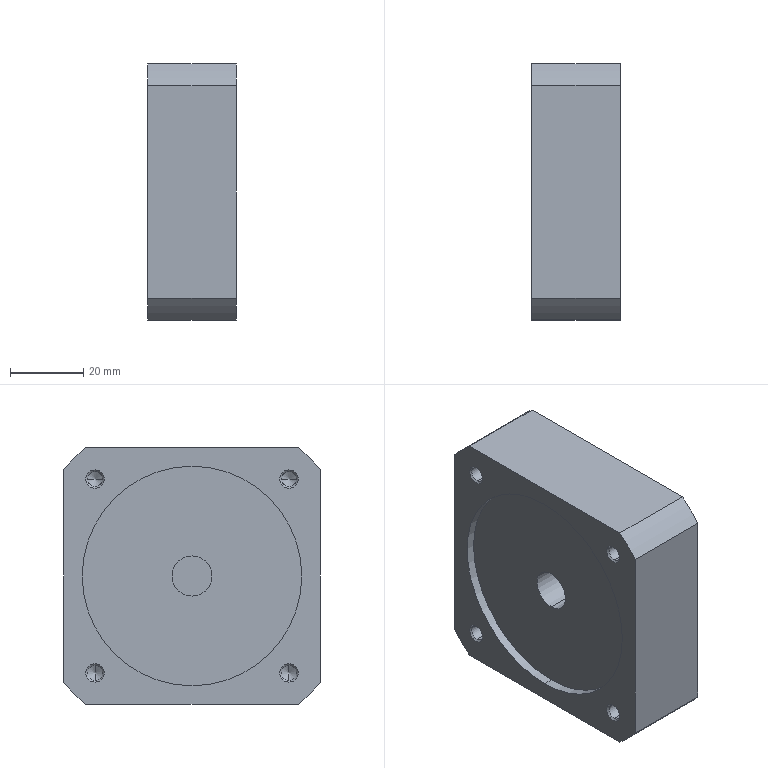Part | STEP file | _PLE60-5_MOTOR-OP2 (intermediate flanges 11-23-60-75-5-70-2.5) | 1 solid | 43 faces | box 24.2 x 70 x 70 mm | volume 107278 mm3 | cylinder 18 | cone 16 | plane 9 | commonest cylinder face diameters 4.134 x8 91 x4 7 x2 11 x2 60 x2
STEP:
#1=CARTESIAN_POINT('',(8.,34.5,5.5));
#2=VERTEX_POINT('',#1);
#3=CARTESIAN_POINT('',(8.,34.5,12.5));
#4=VERTEX_POINT('',#3);
#5=CARTESIAN_POINT('',(8.,34.5,9.));
#6=DIRECTION('',(0.,1.,0.));
#7=DIRECTION('',(0.,0.,1.));
#8=AXIS2_PLACEMENT_3D('',#5,#6,#7);
#9=CIRCLE('',#8,3.5);
#10=EDGE_CURVE('',#2,#4,#9,.T.);
#11=ORIENTED_EDGE('',*,*,#10,.F.);
#12=CARTESIAN_POINT('',(8.,35.,5.5));
#13=VERTEX_POINT('',#12);
#14=CARTESIAN_POINT('',(8.,34.5,5.5));
#15=DIRECTION('',(0.,1.,0.));
#16=VECTOR('',#15,1000.);
#17=LINE('',#14,#16);
#18=EDGE_CURVE('',#2,#13,#17,.T.);
#19=ORIENTED_EDGE('',*,*,#18,.T.);
#20=CARTESIAN_POINT('',(8.,35.,12.5));
#21=VERTEX_POINT('',#20);
#22=CARTESIAN_POINT('',(8.,35.,9.));
#23=DIRECTION('',(0.,1.,0.));
#24=DIRECTION('',(0.,0.,1.));
#25=AXIS2_PLACEMENT_3D('',#22,#23,#24);
#26=CIRCLE('',#25,3.5);
#27=EDGE_CURVE('',#13,#21,#26,.T.);
#28=ORIENTED_EDGE('',*,*,#27,.T.);
#29=CARTESIAN_POINT('',(8.,34.5,12.5));
#30=DIRECTION('',(0.,1.,0.));
#31=VECTOR('',#30,1000.);
#32=LINE('',#29,#31);
#33=EDGE_CURVE('',#4,#21,#32,.T.);
#34=ORIENTED_EDGE('',*,*,#33,.F.);
#35=EDGE_LOOP('',(#11,#19,#28,#34));
#36=FACE_OUTER_BOUND('',#35,.T.);
#37=CARTESIAN_POINT('',(8.,34.5,9.));
#38=DIRECTION('',(0.,1.,0.));
#39=DIRECTION('',(0.,0.,1.));
#40=AXIS2_PLACEMENT_3D('',#37,#38,#39);
#41=CYLINDRICAL_SURFACE('',#40,3.5);
#42=ADVANCED_FACE('',(#36),#41,.F.);
#43=CARTESIAN_POINT('',(2.5,0.,-30.));
#44=VERTEX_POINT('',#43);
#45=CARTESIAN_POINT('',(2.5,0.,30.));
#46=VERTEX_POINT('',#45);
#47=CARTESIAN_POINT('',(2.5,0.,0.));
#48=DIRECTION('',(-1.,0.,0.));
#49=DIRECTION('',(0.,0.,1.));
#50=AXIS2_PLACEMENT_3D('',#47,#48,#49);
#51=CIRCLE('',#50,30.);
#52=EDGE_CURVE('',#44,#46,#51,.T.);
#53=ORIENTED_EDGE('',*,*,#52,.F.);
#54=CARTESIAN_POINT('',(0.,0.,-30.));
#55=VERTEX_POINT('',#54);
#56=CARTESIAN_POINT('',(23.,0.,-30.));
#57=DIRECTION('',(-1.,0.,0.));
#58=VECTOR('',#57,1000.);
#59=LINE('',#56,#58);
#60=EDGE_CURVE('',#44,#55,#59,.T.);
#61=ORIENTED_EDGE('',*,*,#60,.T.);
#62=CARTESIAN_POINT('',(0.,0.,30.));
#63=VERTEX_POINT('',#62);
#64=CARTESIAN_POINT('',(0.,0.,0.));
#65=DIRECTION('',(-1.,0.,0.));
#66=DIRECTION('',(0.,0.,1.));
#67=AXIS2_PLACEMENT_3D('',#64,#65,#66);
#68=CIRCLE('',#67,30.);
#69=EDGE_CURVE('',#55,#63,#68,.T.);
#70=ORIENTED_EDGE('',*,*,#69,.T.);
#71=CARTESIAN_POINT('',(23.,0.,30.));
#72=DIRECTION('',(-1.,0.,0.));
#73=VECTOR('',#72,1000.);
#74=LINE('',#71,#73);
#75=EDGE_CURVE('',#46,#63,#74,.T.);
#76=ORIENTED_EDGE('',*,*,#75,.F.);
#77=EDGE_LOOP('',(#53,#61,#70,#76));
#78=FACE_OUTER_BOUND('',#77,.T.);
#79=CARTESIAN_POINT('',(23.,0.,0.));
#80=DIRECTION('',(-1.,0.,0.));
#81=DIRECTION('',(0.,0.,1.));
#82=AXIS2_PLACEMENT_3D('',#79,#80,#81);
#83=CYLINDRICAL_SURFACE('',#82,30.);
#84=ADVANCED_FACE('',(#78),#83,.F.);
#85=CARTESIAN_POINT('',(0.433,26.517,-28.584));
#86=VERTEX_POINT('',#85);
#87=CARTESIAN_POINT('',(0.433,26.517,-24.45));
#88=VERTEX_POINT('',#87);
#89=CARTESIAN_POINT('',(0.433,26.517,-26.517));
#90=DIRECTION('',(-1.,0.,0.));
#91=DIRECTION('',(0.,0.,1.));
#92=AXIS2_PLACEMENT_3D('',#89,#90,#91);
#93=CIRCLE('',#92,2.067);
#94=EDGE_CURVE('',#86,#88,#93,.T.);
#95=ORIENTED_EDGE('',*,*,#94,.F.);
#96=CARTESIAN_POINT('',(0.,26.517,-29.017));
#97=VERTEX_POINT('',#96);
#98=CARTESIAN_POINT('',(0.,26.517,-29.017));
#99=DIRECTION('',(-0.7071,0.,-0.7071));
#100=VECTOR('',#99,1000.);
#101=LINE('',#98,#100);
#102=EDGE_CURVE('',#86,#97,#101,.T.);
#103=ORIENTED_EDGE('',*,*,#102,.T.);
#104=CARTESIAN_POINT('',(0.,26.517,-24.017));
#105=VERTEX_POINT('',#104);
#106=CARTESIAN_POINT('',(0.,26.517,-26.517));
#107=DIRECTION('',(-1.,0.,0.));
#108=DIRECTION('',(0.,0.,1.));
#109=AXIS2_PLACEMENT_3D('',#106,#107,#108);
#110=CIRCLE('',#109,2.5);
#111=EDGE_CURVE('',#97,#105,#110,.T.);
#112=ORIENTED_EDGE('',*,*,#111,.T.);
#113=CARTESIAN_POINT('',(0.,26.517,-24.017));
#114=DIRECTION('',(-0.7071,0.,0.7071));
#115=VECTOR('',#114,1000.);
#116=LINE('',#113,#115);
#117=EDGE_CURVE('',#88,#105,#116,.T.);
#118=ORIENTED_EDGE('',*,*,#117,.F.);
#119=EDGE_LOOP('',(#95,#103,#112,#118));
#120=FACE_OUTER_BOUND('',#119,.T.);
#121=CARTESIAN_POINT('',(0.,26.517,-26.517));
#122=DIRECTION('',(-1.,0.,0.));
#123=DIRECTION('',(0.,0.,1.));
#124=AXIS2_PLACEMENT_3D('',#121,#122,#123);
#125=CONICAL_SURFACE('',#124,2.5,0.7854);
#126=ADVANCED_FACE('',(#120),#125,.F.);
#127=CARTESIAN_POINT('',(0.433,-26.517,-28.584));
#128=VERTEX_POINT('',#127);
#129=CARTESIAN_POINT('',(0.433,-26.517,-24.45));
#130=VERTEX_POINT('',#129);
#131=CARTESIAN_POINT('',(0.433,-26.517,-26.517));
#132=DIRECTION('',(-1.,0.,0.));
#133=DIRECTION('',(0.,0.,1.));
#134=AXIS2_PLACEMENT_3D('',#131,#132,#133);
#135=CIRCLE('',#134,2.067);
#136=EDGE_CURVE('',#128,#130,#135,.T.);
#137=ORIENTED_EDGE('',*,*,#136,.F.);
#138=CARTESIAN_POINT('',(0.,-26.517,-29.017));
#139=VERTEX_POINT('',#138);
#140=CARTESIAN_POINT('',(0.,-26.517,-29.017));
#141=DIRECTION('',(-0.7071,0.,-0.7071));
#142=VECTOR('',#141,1000.);
#143=LINE('',#140,#142);
#144=EDGE_CURVE('',#128,#139,#143,.T.);
#145=ORIENTED_EDGE('',*,*,#144,.T.);
#146=CARTESIAN_POINT('',(0.,-26.517,-24.017));
#147=VERTEX_POINT('',#146);
#148=CARTESIAN_POINT('',(0.,-26.517,-26.517));
#149=DIRECTION('',(-1.,0.,0.));
#150=DIRECTION('',(0.,0.,1.));
#151=AXIS2_PLACEMENT_3D('',#148,#149,#150);
#152=CIRCLE('',#151,2.5);
#153=EDGE_CURVE('',#139,#147,#152,.T.);
#154=ORIENTED_EDGE('',*,*,#153,.T.);
#155=CARTESIAN_POINT('',(0.,-26.517,-24.017));
#156=DIRECTION('',(-0.7071,0.,0.7071));
#157=VECTOR('',#156,1000.);
#158=LINE('',#155,#157);
#159=EDGE_CURVE('',#130,#147,#158,.T.);
#160=ORIENTED_EDGE('',*,*,#159,.F.);
#161=EDGE_LOOP('',(#137,#145,#154,#160));
#162=FACE_OUTER_BOUND('',#161,.T.);
#163=CARTESIAN_POINT('',(0.,-26.517,-26.517));
#164=DIRECTION('',(-1.,0.,0.));
#165=DIRECTION('',(0.,0.,1.));
#166=AXIS2_PLACEMENT_3D('',#163,#164,#165);
#167=CONICAL_SURFACE('',#166,2.5,0.7854);
#168=ADVANCED_FACE('',(#162),#167,.F.);
#169=CARTESIAN_POINT('',(0.433,-26.517,24.45));
#170=VERTEX_POINT('',#169);
#171=CARTESIAN_POINT('',(0.433,-26.517,28.584));
#172=VERTEX_POINT('',#171);
#173=CARTESIAN_POINT('',(0.433,-26.517,26.517));
#174=DIRECTION('',(-1.,0.,0.));
#175=DIRECTION('',(0.,0.,1.));
#176=AXIS2_PLACEMENT_3D('',#173,#174,#175);
#177=CIRCLE('',#176,2.067);
#178=EDGE_CURVE('',#170,#172,#177,.T.);
#179=ORIENTED_EDGE('',*,*,#178,.F.);
#180=CARTESIAN_POINT('',(0.,-26.517,24.017));
#181=VERTEX_POINT('',#180);
#182=CARTESIAN_POINT('',(0.,-26.517,24.017));
#183=DIRECTION('',(-0.7071,0.,-0.7071));
#184=VECTOR('',#183,1000.);
#185=LINE('',#182,#184);
#186=EDGE_CURVE('',#170,#181,#185,.T.);
#187=ORIENTED_EDGE('',*,*,#186,.T.);
#188=CARTESIAN_POINT('',(0.,-26.517,29.017));
#189=VERTEX_POINT('',#188);
#190=CARTESIAN_POINT('',(0.,-26.517,26.517));
#191=DIRECTION('',(-1.,0.,0.));
#192=DIRECTION('',(0.,0.,1.));
#193=AXIS2_PLACEMENT_3D('',#190,#191,#192);
#194=CIRCLE('',#193,2.5);
#195=EDGE_CURVE('',#181,#189,#194,.T.);
#196=ORIENTED_EDGE('',*,*,#195,.T.);
#197=CARTESIAN_POINT('',(0.,-26.517,29.017));
#198=DIRECTION('',(-0.7071,0.,0.7071));
#199=VECTOR('',#198,1000.);
#200=LINE('',#197,#199);
#201=EDGE_CURVE('',#172,#189,#200,.T.);
#202=ORIENTED_EDGE('',*,*,#201,.F.);
#203=EDGE_LOOP('',(#179,#187,#196,#202));
#204=FACE_OUTER_BOUND('',#203,.T.);
#205=CARTESIAN_POINT('',(0.,-26.517,26.517));
#206=DIRECTION('',(-1.,0.,0.));
#207=DIRECTION('',(0.,0.,1.));
#208=AXIS2_PLACEMENT_3D('',#205,#206,#207);
#209=CONICAL_SURFACE('',#208,2.5,0.7854);
#210=ADVANCED_FACE('',(#204),#209,.F.);
#211=CARTESIAN_POINT('',(0.433,26.517,24.45));
#212=VERTEX_POINT('',#211);
#213=CARTESIAN_POINT('',(0.433,26.517,28.584));
#214=VERTEX_POINT('',#213);
#215=CARTESIAN_POINT('',(0.433,26.517,26.517));
#216=DIRECTION('',(-1.,0.,0.));
#217=DIRECTION('',(0.,0.,1.));
#218=AXIS2_PLACEMENT_3D('',#215,#216,#217);
#219=CIRCLE('',#218,2.067);
#220=EDGE_CURVE('',#212,#214,#219,.T.);
#221=ORIENTED_EDGE('',*,*,#220,.F.);
#222=CARTESIAN_POINT('',(0.,26.517,24.017));
#223=VERTEX_POINT('',#222);
#224=CARTESIAN_POINT('',(0.,26.517,24.017));
#225=DIRECTION('',(-0.7071,0.,-0.7071));
#226=VECTOR('',#225,1000.);
#227=LINE('',#224,#226);
#228=EDGE_CURVE('',#212,#223,#227,.T.);
#229=ORIENTED_EDGE('',*,*,#228,.T.);
#230=CARTESIAN_POINT('',(0.,26.517,29.017));
#231=VERTEX_POINT('',#230);
#232=CARTESIAN_POINT('',(0.,26.517,26.517));
#233=DIRECTION('',(-1.,0.,0.));
#234=DIRECTION('',(0.,0.,1.));
#235=AXIS2_PLACEMENT_3D('',#232,#233,#234);
#236=CIRCLE('',#235,2.5);
#237=EDGE_CURVE('',#223,#231,#236,.T.);
#238=ORIENTED_EDGE('',*,*,#237,.T.);
#239=CARTESIAN_POINT('',(0.,26.517,29.017));
#240=DIRECTION('',(-0.7071,0.,0.7071));
#241=VECTOR('',#240,1000.);
#242=LINE('',#239,#241);
#243=EDGE_CURVE('',#214,#231,#242,.T.);
#244=ORIENTED_EDGE('',*,*,#243,.F.);
#245=EDGE_LOOP('',(#221,#229,#238,#244));
#246=FACE_OUTER_BOUND('',#245,.T.);
#247=CARTESIAN_POINT('',(0.,26.517,26.517));
#248=DIRECTION('',(-1.,0.,0.));
#249=DIRECTION('',(0.,0.,1.));
#250=AXIS2_PLACEMENT_3D('',#247,#248,#249);
#251=CONICAL_SURFACE('',#250,2.5,0.7854);
#252=ADVANCED_FACE('',(#246),#251,.F.);
#253=CARTESIAN_POINT('',(12.,26.517,-28.584));
#254=VERTEX_POINT('',#253);
#255=CARTESIAN_POINT('',(12.,26.517,-24.45));
#256=VERTEX_POINT('',#255);
#257=CARTESIAN_POINT('',(12.,26.517,-26.517));
#258=DIRECTION('',(-1.,0.,0.));
#259=DIRECTION('',(0.,0.,1.));
#260=AXIS2_PLACEMENT_3D('',#257,#258,#259);
#261=CIRCLE('',#260,2.067);
#262=EDGE_CURVE('',#254,#256,#261,.T.);
#263=ORIENTED_EDGE('',*,*,#262,.F.);
#264=CARTESIAN_POINT('',(13.193,26.517,-28.584));
#265=DIRECTION('',(-1.,0.,0.));
#266=VECTOR('',#265,1000.);
#267=LINE('',#264,#266);
#268=EDGE_CURVE('',#254,#86,#267,.T.);
#269=ORIENTED_EDGE('',*,*,#268,.T.);
#270=ORIENTED_EDGE('',*,*,#94,.T.);
#271=CARTESIAN_POINT('',(13.193,26.517,-24.45));
#272=DIRECTION('',(-1.,0.,0.));
#273=VECTOR('',#272,1000.);
#274=LINE('',#271,#273);
#275=EDGE_CURVE('',#256,#88,#274,.T.);
#276=ORIENTED_EDGE('',*,*,#275,.F.);
#277=EDGE_LOOP('',(#263,#269,#270,#276));
#278=FACE_OUTER_BOUND('',#277,.T.);
#279=CARTESIAN_POINT('',(13.193,26.517,-26.517));
#280=DIRECTION('',(-1.,0.,0.));
#281=DIRECTION('',(0.,0.,1.));
#282=AXIS2_PLACEMENT_3D('',#279,#280,#281);
#283=CYLINDRICAL_SURFACE('',#282,2.067);
#284=ADVANCED_FACE('',(#278),#283,.F.);
#285=CARTESIAN_POINT('',(12.,-26.517,-28.584));
#286=VERTEX_POINT('',#285);
#287=CARTESIAN_POINT('',(12.,-26.517,-24.45));
#288=VERTEX_POINT('',#287);
#289=CARTESIAN_POINT('',(12.,-26.517,-26.517));
#290=DIRECTION('',(-1.,0.,0.));
#291=DIRECTION('',(0.,0.,1.));
#292=AXIS2_PLACEMENT_3D('',#289,#290,#291);
#293=CIRCLE('',#292,2.067);
#294=EDGE_CURVE('',#286,#288,#293,.T.);
#295=ORIENTED_EDGE('',*,*,#294,.F.);
#296=CARTESIAN_POINT('',(13.193,-26.517,-28.584));
#297=DIRECTION('',(-1.,0.,0.));
#298=VECTOR('',#297,1000.);
#299=LINE('',#296,#298);
#300=EDGE_CURVE('',#286,#128,#299,.T.);
#301=ORIENTED_EDGE('',*,*,#300,.T.);
#302=ORIENTED_EDGE('',*,*,#136,.T.);
#303=CARTESIAN_POINT('',(13.193,-26.517,-24.45));
#304=DIRECTION('',(-1.,0.,0.));
#305=VECTOR('',#304,1000.);
#306=LINE('',#303,#305);
#307=EDGE_CURVE('',#288,#130,#306,.T.);
#308=ORIENTED_EDGE('',*,*,#307,.F.);
#309=EDGE_LOOP('',(#295,#301,#302,#308));
#310=FACE_OUTER_BOUND('',#309,.T.);
#311=CARTESIAN_POINT('',(13.193,-26.517,-26.517));
#312=DIRECTION('',(-1.,0.,0.));
#313=DIRECTION('',(0.,0.,1.));
#314=AXIS2_PLACEMENT_3D('',#311,#312,#313);
#315=CYLINDRICAL_SURFACE('',#314,2.067);
#316=ADVANCED_FACE('',(#310),#315,.F.);
#317=CARTESIAN_POINT('',(12.,-26.517,24.45));
#318=VERTEX_POINT('',#317);
#319=CARTESIAN_POINT('',(12.,-28.584,26.517));
#320=VERTEX_POINT('',#319);
#321=CARTESIAN_POINT('',(12.,-26.517,26.517));
#322=DIRECTION('',(-1.,0.,0.));
#323=DIRECTION('',(0.,0.,1.));
#324=AXIS2_PLACEMENT_3D('',#321,#322,#323);
#325=CIRCLE('',#324,2.067);
#326=EDGE_CURVE('',#318,#320,#325,.T.);
#327=ORIENTED_EDGE('',*,*,#326,.F.);
#328=CARTESIAN_POINT('',(13.193,-26.517,24.45));
#329=DIRECTION('',(-1.,0.,0.));
#330=VECTOR('',#329,1000.);
#331=LINE('',#328,#330);
#332=EDGE_CURVE('',#318,#170,#331,.T.);
#333=ORIENTED_EDGE('',*,*,#332,.T.);
#334=ORIENTED_EDGE('',*,*,#178,.T.);
#335=CARTESIAN_POINT('',(12.,-26.517,28.584));
#336=VERTEX_POINT('',#335);
#337=CARTESIAN_POINT('',(13.193,-26.517,28.584));
#338=DIRECTION('',(-1.,0.,0.));
#339=VECTOR('',#338,1000.);
#340=LINE('',#337,#339);
#341=EDGE_CURVE('',#336,#172,#340,.T.);
#342=ORIENTED_EDGE('',*,*,#341,.F.);
#343=CARTESIAN_POINT('',(12.,-26.517,26.517));
#344=DIRECTION('',(-1.,0.,0.));
#345=DIRECTION('',(0.,0.,1.));
#346=AXIS2_PLACEMENT_3D('',#343,#344,#345);
#347=CIRCLE('',#346,2.067);
#348=EDGE_CURVE('',#320,#336,#347,.T.);
#349=ORIENTED_EDGE('',*,*,#348,.F.);
#350=EDGE_LOOP('',(#327,#333,#334,#342,#349));
#351=FACE_OUTER_BOUND('',#350,.T.);
#352=CARTESIAN_POINT('',(13.193,-26.517,26.517));
#353=DIRECTION('',(-1.,0.,0.));
#354=DIRECTION('',(0.,0.,1.));
#355=AXIS2_PLACEMENT_3D('',#352,#353,#354);
#356=CYLINDRICAL_SURFACE('',#355,2.067);
#357=ADVANCED_FACE('',(#351),#356,.F.);
#358=CARTESIAN_POINT('',(12.,26.517,24.45));
#359=VERTEX_POINT('',#358);
#360=CARTESIAN_POINT('',(12.,24.45,26.517));
#361=VERTEX_POINT('',#360);
#362=CARTESIAN_POINT('',(12.,26.517,26.517));
#363=DIRECTION('',(-1.,0.,0.));
#364=DIRECTION('',(0.,0.,1.));
#365=AXIS2_PLACEMENT_3D('',#362,#363,#364);
#366=CIRCLE('',#365,2.067);
#367=EDGE_CURVE('',#359,#361,#366,.T.);
#368=ORIENTED_EDGE('',*,*,#367,.F.);
#369=CARTESIAN_POINT('',(13.193,26.517,24.45));
#370=DIRECTION('',(-1.,0.,0.));
#371=VECTOR('',#370,1000.);
#372=LINE('',#369,#371);
#373=EDGE_CURVE('',#359,#212,#372,.T.);
#374=ORIENTED_EDGE('',*,*,#373,.T.);
#375=ORIENTED_EDGE('',*,*,#220,.T.);
#376=CARTESIAN_POINT('',(12.,26.517,28.584));
#377=VERTEX_POINT('',#376);
#378=CARTESIAN_POINT('',(13.193,26.517,28.584));
#379=DIRECTION('',(-1.,0.,0.));
#380=VECTOR('',#379,1000.);
#381=LINE('',#378,#380);
#382=EDGE_CURVE('',#377,#214,#381,.T.);
#383=ORIENTED_EDGE('',*,*,#382,.F.);
#384=CARTESIAN_POINT('',(12.,26.517,26.517));
#385=DIRECTION('',(-1.,0.,0.));
#386=DIRECTION('',(0.,0.,1.));
#387=AXIS2_PLACEMENT_3D('',#384,#385,#386);
#388=CIRCLE('',#387,2.067);
#389=EDGE_CURVE('',#361,#377,#388,.T.);
#390=ORIENTED_EDGE('',*,*,#389,.F.);
#391=EDGE_LOOP('',(#368,#374,#375,#383,#390));
#392=FACE_OUTER_BOUND('',#391,.T.);
#393=CARTESIAN_POINT('',(13.193,26.517,26.517));
#394=DIRECTION('',(-1.,0.,0.));
#395=DIRECTION('',(0.,0.,1.));
#396=AXIS2_PLACEMENT_3D('',#393,#394,#395);
#397=CYLINDRICAL_SURFACE('',#396,2.067);
#398=ADVANCED_FACE('',(#392),#397,.F.);
#399=CARTESIAN_POINT('',(23.,0.,-5.5));
#400=VERTEX_POINT('',#399);
#401=CARTESIAN_POINT('',(23.,0.,5.5));
#402=VERTEX_POINT('',#401);
#403=CARTESIAN_POINT('',(23.,0.,0.));
#404=DIRECTION('',(-1.,0.,0.));
#405=DIRECTION('',(0.,0.,1.));
#406=AXIS2_PLACEMENT_3D('',#403,#404,#405);
#407=CIRCLE('',#406,5.5);
#408=EDGE_CURVE('',#400,#402,#407,.T.);
#409=ORIENTED_EDGE('',*,*,#408,.F.);
#410=CARTESIAN_POINT('',(2.5,0.,-5.5));
#411=VERTEX_POINT('',#410);
#412=CARTESIAN_POINT('',(23.,0.,-5.5));
#413=DIRECTION('',(-1.,0.,0.));
#414=VECTOR('',#413,1000.);
#415=LINE('',#412,#414);
#416=EDGE_CURVE('',#400,#411,#415,.T.);
#417=ORIENTED_EDGE('',*,*,#416,.T.);
#418=CARTESIAN_POINT('',(2.5,0.,5.5));
#419=VERTEX_POINT('',#418);
#420=CARTESIAN_POINT('',(2.5,0.,0.));
#421=DIRECTION('',(1.,0.,0.));
#422=DIRECTION('',(0.,0.,1.));
#423=AXIS2_PLACEMENT_3D('',#420,#421,#422);
#424=CIRCLE('',#423,5.5);
#425=EDGE_CURVE('',#419,#411,#424,.T.);
#426=ORIENTED_EDGE('',*,*,#425,.F.);
#427=CARTESIAN_POINT('',(23.,0.,5.5));
#428=DIRECTION('',(-1.,0.,0.));
#429=VECTOR('',#428,1000.);
#430=LINE('',#427,#429);
#431=EDGE_CURVE('',#402,#419,#430,.T.);
#432=ORIENTED_EDGE('',*,*,#431,.F.);
#433=EDGE_LOOP('',(#409,#417,#426,#432));
#434=FACE_OUTER_BOUND('',#433,.T.);
#435=CARTESIAN_POINT('',(23.,0.,0.));
#436=DIRECTION('',(-1.,0.,0.));
#437=DIRECTION('',(0.,0.,1.));
#438=AXIS2_PLACEMENT_3D('',#435,#436,#437);
#439=CYLINDRICAL_SURFACE('',#438,5.5);
#440=ADVANCED_FACE('',(#434),#439,.F.);
#441=CARTESIAN_POINT('',(13.193,26.517,-26.517));
#442=VERTEX_POINT('',#441);
#443=CARTESIAN_POINT('',(12.,26.517,-24.45));
#444=DIRECTION('',(-0.5,0.,0.866));
#445=VECTOR('',#444,1000.);
#446=LINE('',#443,#445);
#447=EDGE_CURVE('',#442,#256,#446,.T.);
#448=ORIENTED_EDGE('',*,*,#447,.F.);
#449=CARTESIAN_POINT('',(12.,26.517,-28.584));
#450=DIRECTION('',(-0.5,0.,-0.866));
#451=VECTOR('',#450,1000.);
#452=LINE('',#449,#451);
#453=EDGE_CURVE('',#442,#254,#452,.T.);
#454=ORIENTED_EDGE('',*,*,#453,.T.);
#455=ORIENTED_EDGE('',*,*,#262,.T.);
#456=EDGE_LOOP('',(#448,#454,#455));
#457=FACE_OUTER_BOUND('',#456,.T.);
#458=CARTESIAN_POINT('',(12.,26.517,-26.517));
#459=DIRECTION('',(-1.,0.,0.));
#460=DIRECTION('',(0.,0.,1.));
#461=AXIS2_PLACEMENT_3D('',#458,#459,#460);
#462=CONICAL_SURFACE('',#461,2.067,1.047);
#463=ADVANCED_FACE('',(#457),#462,.F.);
#464=CARTESIAN_POINT('',(13.193,-26.517,-26.517));
#465=VERTEX_POINT('',#464);
#466=CARTESIAN_POINT('',(12.,-26.517,-24.45));
#467=DIRECTION('',(-0.5,0.,0.866));
#468=VECTOR('',#467,1000.);
#469=LINE('',#466,#468);
#470=EDGE_CURVE('',#465,#288,#469,.T.);
#471=ORIENTED_EDGE('',*,*,#470,.F.);
#472=CARTESIAN_POINT('',(12.,-26.517,-28.584));
#473=DIRECTION('',(-0.5,0.,-0.866));
#474=VECTOR('',#473,1000.);
#475=LINE('',#472,#474);
#476=EDGE_CURVE('',#465,#286,#475,.T.);
#477=ORIENTED_EDGE('',*,*,#476,.T.);
#478=ORIENTED_EDGE('',*,*,#294,.T.);
#479=EDGE_LOOP('',(#471,#477,#478));
#480=FACE_OUTER_BOUND('',#479,.T.);
#481=CARTESIAN_POINT('',(12.,-26.517,-26.517));
#482=DIRECTION('',(-1.,0.,0.));
#483=DIRECTION('',(0.,0.,1.));
#484=AXIS2_PLACEMENT_3D('',#481,#482,#483);
#485=CONICAL_SURFACE('',#484,2.067,1.047);
#486=ADVANCED_FACE('',(#480),#485,.F.);
#487=CARTESIAN_POINT('',(13.193,-26.517,26.517));
#488=VERTEX_POINT('',#487);
#489=CARTESIAN_POINT('',(12.,-28.584,26.517));
#490=DIRECTION('',(-0.5,-0.866,0.));
#491=VECTOR('',#490,1000.);
#492=LINE('',#489,#491);
#493=EDGE_CURVE('',#488,#320,#492,.T.);
#494=ORIENTED_EDGE('',*,*,#493,.F.);
#495=CARTESIAN_POINT('',(12.,-24.45,26.517));
#496=VERTEX_POINT('',#495);
#497=CARTESIAN_POINT('',(12.,-24.45,26.517));
#498=DIRECTION('',(-0.5,0.866,0.));
#499=VECTOR('',#498,1000.);
#500=LINE('',#497,#499);
#501=EDGE_CURVE('',#488,#496,#500,.T.);
#502=ORIENTED_EDGE('',*,*,#501,.T.);
#503=CARTESIAN_POINT('',(12.,-26.517,26.517));
#504=DIRECTION('',(-1.,0.,0.));
#505=DIRECTION('',(0.,0.,1.));
#506=AXIS2_PLACEMENT_3D('',#503,#504,#505);
#507=CIRCLE('',#506,2.067);
#508=EDGE_CURVE('',#496,#318,#507,.T.);
#509=ORIENTED_EDGE('',*,*,#508,.T.);
#510=ORIENTED_EDGE('',*,*,#326,.T.);
#511=EDGE_LOOP('',(#494,#502,#509,#510));
#512=FACE_OUTER_BOUND('',#511,.T.);
#513=CARTESIAN_POINT('',(12.,-26.517,26.517));
#514=DIRECTION('',(-1.,0.,0.));
#515=DIRECTION('',(0.,-1.,0.));
#516=AXIS2_PLACEMENT_3D('',#513,#514,#515);
#517=CONICAL_SURFACE('',#516,2.067,1.047);
#518=ADVANCED_FACE('',(#512),#517,.F.);
#519=CARTESIAN_POINT('',(13.193,26.517,26.517));
#520=VERTEX_POINT('',#519);
#521=CARTESIAN_POINT('',(12.,24.45,26.517));
#522=DIRECTION('',(-0.5,-0.866,0.));
#523=VECTOR('',#522,1000.);
#524=LINE('',#521,#523);
#525=EDGE_CURVE('',#520,#361,#524,.T.);
#526=ORIENTED_EDGE('',*,*,#525,.F.);
#527=CARTESIAN_POINT('',(12.,28.584,26.517));
#528=VERTEX_POINT('',#527);
#529=CARTESIAN_POINT('',(12.,28.584,26.517));
#530=DIRECTION('',(-0.5,0.866,0.));
#531=VECTOR('',#530,1000.);
#532=LINE('',#529,#531);
#533=EDGE_CURVE('',#520,#528,#532,.T.);
#534=ORIENTED_EDGE('',*,*,#533,.T.);
#535=CARTESIAN_POINT('',(12.,26.517,26.517));
#536=DIRECTION('',(-1.,0.,0.));
#537=DIRECTION('',(0.,0.,1.));
#538=AXIS2_PLACEMENT_3D('',#535,#536,#537);
#539=CIRCLE('',#538,2.067);
#540=EDGE_CURVE('',#528,#359,#539,.T.);
#541=ORIENTED_EDGE('',*,*,#540,.T.);
#542=ORIENTED_EDGE('',*,*,#367,.T.);
#543=EDGE_LOOP('',(#526,#534,#541,#542));
#544=FACE_OUTER_BOUND('',#543,.T.);
#545=CARTESIAN_POINT('',(12.,26.517,26.517));
#546=DIRECTION('',(-1.,0.,0.));
#547=DIRECTION('',(0.,-1.,0.));
#548=AXIS2_PLACEMENT_3D('',#545,#546,#547);
#549=CONICAL_SURFACE('',#548,2.067,1.047);
#550=ADVANCED_FACE('',(#544),#549,.F.);
#551=CARTESIAN_POINT('',(24.2,35.,-29.073));
#552=VERTEX_POINT('',#551);
#553=CARTESIAN_POINT('',(24.2,35.,29.073));
#554=VERTEX_POINT('',#553);
#555=CARTESIAN_POINT('',(24.2,35.,0.));
#556=DIRECTION('',(0.,0.,1.));
#557=VECTOR('',#556,1000.);
#558=LINE('',#555,#557);
#559=EDGE_CURVE('',#552,#554,#558,.T.);
#560=ORIENTED_EDGE('',*,*,#559,.T.);
#561=CARTESIAN_POINT('',(24.2,29.073,35.));
#562=VERTEX_POINT('',#561);
#563=CARTESIAN_POINT('',(24.2,0.,0.));
#564=DIRECTION('',(1.,0.,0.));
#565=DIRECTION('',(0.,0.,-1.));
#566=AXIS2_PLACEMENT_3D('',#563,#564,#565);
#567=CIRCLE('',#566,45.5);
#568=EDGE_CURVE('',#554,#562,#567,.T.);
#569=ORIENTED_EDGE('',*,*,#568,.T.);
#570=CARTESIAN_POINT('',(24.2,-29.073,35.));
#571=VERTEX_POINT('',#570);
#572=CARTESIAN_POINT('',(24.2,0.,35.));
#573=DIRECTION('',(0.,-1.,0.));
#574=VECTOR('',#573,1000.);
#575=LINE('',#572,#574);
#576=EDGE_CURVE('',#562,#571,#575,.T.);
#577=ORIENTED_EDGE('',*,*,#576,.T.);
#578=CARTESIAN_POINT('',(24.2,-35.,29.073));
#579=VERTEX_POINT('',#578);
#580=CARTESIAN_POINT('',(24.2,0.,0.));
#581=DIRECTION('',(1.,0.,0.));
#582=DIRECTION('',(0.,0.,-1.));
#583=AXIS2_PLACEMENT_3D('',#580,#581,#582);
#584=CIRCLE('',#583,45.5);
#585=EDGE_CURVE('',#571,#579,#584,.T.);
#586=ORIENTED_EDGE('',*,*,#585,.T.);
#587=CARTESIAN_POINT('',(24.2,-35.,-29.073));
#588=VERTEX_POINT('',#587);
#589=CARTESIAN_POINT('',(24.2,-35.,0.));
#590=DIRECTION('',(0.,0.,-1.));
#591=VECTOR('',#590,1000.);
#592=LINE('',#589,#591);
#593=EDGE_CURVE('',#579,#588,#592,.T.);
#594=ORIENTED_EDGE('',*,*,#593,.T.);
#595=CARTESIAN_POINT('',(24.2,-29.073,-35.));
#596=VERTEX_POINT('',#595);
#597=CARTESIAN_POINT('',(24.2,0.,0.));
#598=DIRECTION('',(1.,0.,0.));
#599=DIRECTION('',(0.,0.,-1.));
#600=AXIS2_PLACEMENT_3D('',#597,#598,#599);
#601=CIRCLE('',#600,45.5);
#602=EDGE_CURVE('',#588,#596,#601,.T.);
#603=ORIENTED_EDGE('',*,*,#602,.T.);
#604=CARTESIAN_POINT('',(24.2,29.073,-35.));
#605=VERTEX_POINT('',#604);
#606=CARTESIAN_POINT('',(24.2,0.,-35.));
#607=DIRECTION('',(0.,1.,0.));
#608=VECTOR('',#607,1000.);
#609=LINE('',#606,#608);
#610=EDGE_CURVE('',#596,#605,#609,.T.);
#611=ORIENTED_EDGE('',*,*,#610,.T.);
#612=CARTESIAN_POINT('',(24.2,0.,0.));
#613=DIRECTION('',(1.,0.,0.));
#614=DIRECTION('',(0.,0.,-1.));
#615=AXIS2_PLACEMENT_3D('',#612,#613,#614);
#616=CIRCLE('',#615,45.5);
#617=EDGE_CURVE('',#605,#552,#616,.T.);
#618=ORIENTED_EDGE('',*,*,#617,.T.);
#619=EDGE_LOOP('',(#560,#569,#577,#586,#594,#603,#611,#618));
#620=FACE_OUTER_BOUND('',#619,.T.);
#621=CARTESIAN_POINT('',(24.2,0.,0.));
#622=DIRECTION('',(1.,0.,0.));
#623=DIRECTION('',(0.,0.,-1.));
#624=AXIS2_PLACEMENT_3D('',#621,#622,#623);
#625=PLANE('',#624);
#626=ADVANCED_FACE('',(#620),#625,.T.);
#627=ORIENTED_EDGE('',*,*,#568,.F.);
#628=CARTESIAN_POINT('',(0.,35.,29.073));
#629=VERTEX_POINT('',#628);
#630=CARTESIAN_POINT('',(24.2,35.,29.073));
#631=DIRECTION('',(-1.,0.,0.));
#632=VECTOR('',#631,1000.);
#633=LINE('',#630,#632);
#634=EDGE_CURVE('',#554,#629,#633,.T.);
#635=ORIENTED_EDGE('',*,*,#634,.T.);
#636=CARTESIAN_POINT('',(0.,29.073,35.));
#637=VERTEX_POINT('',#636);
#638=CARTESIAN_POINT('',(0.,0.,0.));
#639=DIRECTION('',(1.,0.,0.));
#640=DIRECTION('',(0.,0.,-1.));
#641=AXIS2_PLACEMENT_3D('',#638,#639,#640);
#642=CIRCLE('',#641,45.5);
#643=EDGE_CURVE('',#629,#637,#642,.T.);
#644=ORIENTED_EDGE('',*,*,#643,.T.);
#645=CARTESIAN_POINT('',(24.2,29.073,35.));
#646=DIRECTION('',(1.,0.,0.));
#647=VECTOR('',#646,1000.);
#648=LINE('',#645,#647);
#649=EDGE_CURVE('',#637,#562,#648,.T.);
#650=ORIENTED_EDGE('',*,*,#649,.T.);
#651=EDGE_LOOP('',(#627,#635,#644,#650));
#652=FACE_OUTER_BOUND('',#651,.T.);
#653=CARTESIAN_POINT('',(24.2,0.,0.));
#654=DIRECTION('',(1.,0.,0.));
#655=DIRECTION('',(0.,0.,-1.));
#656=AXIS2_PLACEMENT_3D('',#653,#654,#655);
#657=CYLINDRICAL_SURFACE('',#656,45.5);
#658=ADVANCED_FACE('',(#652),#657,.T.);
#659=ORIENTED_EDGE('',*,*,#634,.F.);
#660=ORIENTED_EDGE('',*,*,#559,.F.);
#661=CARTESIAN_POINT('',(0.,35.,-29.073));
#662=VERTEX_POINT('',#661);
#663=CARTESIAN_POINT('',(24.2,35.,-29.073));
#664=DIRECTION('',(1.,0.,0.));
#665=VECTOR('',#664,1000.);
#666=LINE('',#663,#665);
#667=EDGE_CURVE('',#662,#552,#666,.T.);
#668=ORIENTED_EDGE('',*,*,#667,.F.);
#669=CARTESIAN_POINT('',(0.,35.,-29.073));
#670=DIRECTION('',(0.,0.,-1.));
#671=VECTOR('',#670,1000.);
#672=LINE('',#669,#671);
#673=EDGE_CURVE('',#629,#662,#672,.T.);
#674=ORIENTED_EDGE('',*,*,#673,.F.);
#675=EDGE_LOOP('',(#659,#660,#668,#674));
#676=FACE_OUTER_BOUND('',#675,.T.);
#677=CARTESIAN_POINT('',(8.,35.,9.));
#678=DIRECTION('',(0.,1.,0.));
#679=DIRECTION('',(0.,0.,1.));
#680=AXIS2_PLACEMENT_3D('',#677,#678,#679);
#681=CIRCLE('',#680,3.5);
#682=EDGE_CURVE('',#21,#13,#681,.T.);
#683=ORIENTED_EDGE('',*,*,#682,.F.);
#684=ORIENTED_EDGE('',*,*,#27,.F.);
#685=EDGE_LOOP('',(#683,#684));
#686=FACE_BOUND('',#685,.T.);
#687=CARTESIAN_POINT('',(24.2,35.,-29.073));
#688=DIRECTION('',(0.,-1.,0.));
#689=DIRECTION('',(0.,0.,-1.));
#690=AXIS2_PLACEMENT_3D('',#687,#688,#689);
#691=PLANE('',#690);
#692=ADVANCED_FACE('',(#676,#686),#691,.F.);
#693=ORIENTED_EDGE('',*,*,#617,.F.);
#694=CARTESIAN_POINT('',(0.,29.073,-35.));
#695=VERTEX_POINT('',#694);
#696=CARTESIAN_POINT('',(24.2,29.073,-35.));
#697=DIRECTION('',(-1.,0.,0.));
#698=VECTOR('',#697,1000.);
#699=LINE('',#696,#698);
#700=EDGE_CURVE('',#605,#695,#699,.T.);
#701=ORIENTED_EDGE('',*,*,#700,.T.);
#702=CARTESIAN_POINT('',(0.,0.,0.));
#703=DIRECTION('',(1.,0.,0.));
#704=DIRECTION('',(0.,0.,-1.));
#705=AXIS2_PLACEMENT_3D('',#702,#703,#704);
#706=CIRCLE('',#705,45.5);
#707=EDGE_CURVE('',#695,#662,#706,.T.);
#708=ORIENTED_EDGE('',*,*,#707,.T.);
#709=ORIENTED_EDGE('',*,*,#667,.T.);
#710=EDGE_LOOP('',(#693,#701,#708,#709));
#711=FACE_OUTER_BOUND('',#710,.T.);
#712=CARTESIAN_POINT('',(24.2,0.,0.));
#713=DIRECTION('',(1.,0.,0.));
#714=DIRECTION('',(0.,0.,-1.));
#715=AXIS2_PLACEMENT_3D('',#712,#713,#714);
#716=CYLINDRICAL_SURFACE('',#715,45.5);
#717=ADVANCED_FACE('',(#711),#716,.T.);
#718=ORIENTED_EDGE('',*,*,#700,.F.);
#719=ORIENTED_EDGE('',*,*,#610,.F.);
#720=CARTESIAN_POINT('',(0.,-29.073,-35.));
#721=VERTEX_POINT('',#720);
#722=CARTESIAN_POINT('',(24.2,-29.073,-35.));
#723=DIRECTION('',(1.,0.,0.));
#724=VECTOR('',#723,1000.);
#725=LINE('',#722,#724);
#726=EDGE_CURVE('',#721,#596,#725,.T.);
#727=ORIENTED_EDGE('',*,*,#726,.F.);
#728=CARTESIAN_POINT('',(0.,-29.073,-35.));
#729=DIRECTION('',(0.,-1.,0.));
#730=VECTOR('',#729,1000.);
#731=LINE('',#728,#730);
#732=EDGE_CURVE('',#695,#721,#731,.T.);
#733=ORIENTED_EDGE('',*,*,#732,.F.);
#734=EDGE_LOOP('',(#718,#719,#727,#733));
#735=FACE_OUTER_BOUND('',#734,.T.);
#736=CARTESIAN_POINT('',(24.2,-29.073,-35.));
#737=DIRECTION('',(0.,0.,1.));
#738=DIRECTION('',(1.,0.,0.));
#739=AXIS2_PLACEMENT_3D('',#736,#737,#738);
#740=PLANE('',#739);
#741=ADVANCED_FACE('',(#735),#740,.F.);
#742=ORIENTED_EDGE('',*,*,#602,.F.);
#743=CARTESIAN_POINT('',(0.,-35.,-29.073));
#744=VERTEX_POINT('',#743);
#745=CARTESIAN_POINT('',(24.2,-35.,-29.073));
#746=DIRECTION('',(-1.,0.,0.));
#747=VECTOR('',#746,1000.);
#748=LINE('',#745,#747);
#749=EDGE_CURVE('',#588,#744,#748,.T.);
#750=ORIENTED_EDGE('',*,*,#749,.T.);
#751=CARTESIAN_POINT('',(0.,0.,0.));
#752=DIRECTION('',(1.,0.,0.));
#753=DIRECTION('',(0.,0.,-1.));
#754=AXIS2_PLACEMENT_3D('',#751,#752,#753);
#755=CIRCLE('',#754,45.5);
#756=EDGE_CURVE('',#744,#721,#755,.T.);
#757=ORIENTED_EDGE('',*,*,#756,.T.);
#758=ORIENTED_EDGE('',*,*,#726,.T.);
#759=EDGE_LOOP('',(#742,#750,#757,#758));
#760=FACE_OUTER_BOUND('',#759,.T.);
#761=CARTESIAN_POINT('',(24.2,0.,0.));
#762=DIRECTION('',(1.,0.,0.));
#763=DIRECTION('',(0.,0.,-1.));
#764=AXIS2_PLACEMENT_3D('',#761,#762,#763);
#765=CYLINDRICAL_SURFACE('',#764,45.5);
#766=ADVANCED_FACE('',(#760),#765,.T.);
#767=ORIENTED_EDGE('',*,*,#749,.F.);
#768=ORIENTED_EDGE('',*,*,#593,.F.);
#769=CARTESIAN_POINT('',(0.,-35.,29.073));
#770=VERTEX_POINT('',#769);
#771=CARTESIAN_POINT('',(24.2,-35.,29.073));
#772=DIRECTION('',(1.,0.,0.));
#773=VECTOR('',#772,1000.);
#774=LINE('',#771,#773);
#775=EDGE_CURVE('',#770,#579,#774,.T.);
#776=ORIENTED_EDGE('',*,*,#775,.F.);
#777=CARTESIAN_POINT('',(0.,-35.,29.073));
#778=DIRECTION('',(0.,0.,1.));
#779=VECTOR('',#778,1000.);
#780=LINE('',#777,#779);
#781=EDGE_CURVE('',#744,#770,#780,.T.);
#782=ORIENTED_EDGE('',*,*,#781,.F.);
#783=EDGE_LOOP('',(#767,#768,#776,#782));
#784=FACE_OUTER_BOUND('',#783,.T.);
#785=CARTESIAN_POINT('',(24.2,-35.,29.073));
#786=DIRECTION('',(0.,1.,0.));
#787=DIRECTION('',(0.,0.,1.));
#788=AXIS2_PLACEMENT_3D('',#785,#786,#787);
#789=PLANE('',#788);
#790=ADVANCED_FACE('',(#784),#789,.F.);
#791=ORIENTED_EDGE('',*,*,#585,.F.);
#792=CARTESIAN_POINT('',(0.,-29.073,35.));
#793=VERTEX_POINT('',#792);
#794=CARTESIAN_POINT('',(24.2,-29.073,35.));
#795=DIRECTION('',(-1.,0.,0.));
#796=VECTOR('',#795,1000.);
#797=LINE('',#794,#796);
#798=EDGE_CURVE('',#571,#793,#797,.T.);
#799=ORIENTED_EDGE('',*,*,#798,.T.);
#800=CARTESIAN_POINT('',(0.,0.,0.));
#801=DIRECTION('',(1.,0.,0.));
#802=DIRECTION('',(0.,0.,-1.));
#803=AXIS2_PLACEMENT_3D('',#800,#801,#802);
#804=CIRCLE('',#803,45.5);
#805=EDGE_CURVE('',#793,#770,#804,.T.);
#806=ORIENTED_EDGE('',*,*,#805,.T.);
#807=ORIENTED_EDGE('',*,*,#775,.T.);
#808=EDGE_LOOP('',(#791,#799,#806,#807));
#809=FACE_OUTER_BOUND('',#808,.T.);
#810=CARTESIAN_POINT('',(24.2,0.,0.));
#811=DIRECTION('',(1.,0.,0.));
#812=DIRECTION('',(0.,0.,-1.));
#813=AXIS2_PLACEMENT_3D('',#810,#811,#812);
#814=CYLINDRICAL_SURFACE('',#813,45.5);
#815=ADVANCED_FACE('',(#809),#814,.T.);
#816=ORIENTED_EDGE('',*,*,#798,.F.);
#817=ORIENTED_EDGE('',*,*,#576,.F.);
#818=ORIENTED_EDGE('',*,*,#649,.F.);
#819=CARTESIAN_POINT('',(0.,29.073,35.));
#820=DIRECTION('',(0.,1.,0.));
#821=VECTOR('',#820,1000.);
#822=LINE('',#819,#821);
#823=EDGE_CURVE('',#793,#637,#822,.T.);
#824=ORIENTED_EDGE('',*,*,#823,.F.);
#825=EDGE_LOOP('',(#816,#817,#818,#824));
#826=FACE_OUTER_BOUND('',#825,.T.);
#827=CARTESIAN_POINT('',(24.2,29.073,35.));
#828=DIRECTION('',(0.,0.,-1.));
#829=DIRECTION('',(-1.,0.,0.));
#830=AXIS2_PLACEMENT_3D('',#827,#828,#829);
#831=PLANE('',#830);
#832=ADVANCED_FACE('',(#826),#831,.F.);
#833=ORIENTED_EDGE('',*,*,#643,.F.);
#834=ORIENTED_EDGE('',*,*,#673,.T.);
#835=ORIENTED_EDGE('',*,*,#707,.F.);
#836=ORIENTED_EDGE('',*,*,#732,.T.);
#837=ORIENTED_EDGE('',*,*,#756,.F.);
#838=ORIENTED_EDGE('',*,*,#781,.T.);
#839=ORIENTED_EDGE('',*,*,#805,.F.);
#840=ORIENTED_EDGE('',*,*,#823,.T.);
#841=EDGE_LOOP('',(#833,#834,#835,#836,#837,#838,#839,#840));
#842=FACE_OUTER_BOUND('',#841,.T.);
#843=CARTESIAN_POINT('',(0.,0.,0.));
#844=DIRECTION('',(-1.,0.,0.));
#845=DIRECTION('',(0.,0.,1.));
#846=AXIS2_PLACEMENT_3D('',#843,#844,#845);
#847=CIRCLE('',#846,30.);
#848=EDGE_CURVE('',#63,#55,#847,.T.);
#849=ORIENTED_EDGE('',*,*,#848,.F.);
#850=ORIENTED_EDGE('',*,*,#69,.F.);
#851=EDGE_LOOP('',(#849,#850));
#852=FACE_BOUND('',#851,.T.);
#853=CARTESIAN_POINT('',(0.,26.517,-26.517));
#854=DIRECTION('',(-1.,0.,0.));
#855=DIRECTION('',(0.,0.,1.));
#856=AXIS2_PLACEMENT_3D('',#853,#854,#855);
#857=CIRCLE('',#856,2.5);
#858=EDGE_CURVE('',#105,#97,#857,.T.);
#859=ORIENTED_EDGE('',*,*,#858,.F.);
#860=ORIENTED_EDGE('',*,*,#111,.F.);
#861=EDGE_LOOP('',(#859,#860));
#862=FACE_BOUND('',#861,.T.);
#863=CARTESIAN_POINT('',(0.,-26.517,-26.517));
#864=DIRECTION('',(-1.,0.,0.));
#865=DIRECTION('',(0.,0.,1.));
#866=AXIS2_PLACEMENT_3D('',#863,#864,#865);
#867=CIRCLE('',#866,2.5);
#868=EDGE_CURVE('',#147,#139,#867,.T.);
#869=ORIENTED_EDGE('',*,*,#868,.F.);
#870=ORIENTED_EDGE('',*,*,#153,.F.);
#871=EDGE_LOOP('',(#869,#870));
#872=FACE_BOUND('',#871,.T.);
#873=CARTESIAN_POINT('',(0.,-26.517,26.517));
#874=DIRECTION('',(-1.,0.,0.));
#875=DIRECTION('',(0.,0.,1.));
#876=AXIS2_PLACEMENT_3D('',#873,#874,#875);
#877=CIRCLE('',#876,2.5);
#878=EDGE_CURVE('',#189,#181,#877,.T.);
#879=ORIENTED_EDGE('',*,*,#878,.F.);
#880=ORIENTED_EDGE('',*,*,#195,.F.);
#881=EDGE_LOOP('',(#879,#880));
#882=FACE_BOUND('',#881,.T.);
#883=CARTESIAN_POINT('',(0.,26.517,26.517));
#884=DIRECTION('',(-1.,0.,0.));
#885=DIRECTION('',(0.,0.,1.));
#886=AXIS2_PLACEMENT_3D('',#883,#884,#885);
#887=CIRCLE('',#886,2.5);
#888=EDGE_CURVE('',#231,#223,#887,.T.);
#889=ORIENTED_EDGE('',*,*,#888,.F.);
#890=ORIENTED_EDGE('',*,*,#237,.F.);
#891=EDGE_LOOP('',(#889,#890));
#892=FACE_BOUND('',#891,.T.);
#893=CARTESIAN_POINT('',(0.,0.,0.));
#894=DIRECTION('',(1.,0.,0.));
#895=DIRECTION('',(0.,0.,-1.));
#896=AXIS2_PLACEMENT_3D('',#893,#894,#895);
#897=PLANE('',#896);
#898=ADVANCED_FACE('',(#842,#852,#862,#872,#882,#892),#897,.F.);
#899=ORIENTED_EDGE('',*,*,#18,.F.);
#900=CARTESIAN_POINT('',(8.,34.5,9.));
#901=DIRECTION('',(0.,1.,0.));
#902=DIRECTION('',(0.,0.,1.));
#903=AXIS2_PLACEMENT_3D('',#900,#901,#902);
#904=CIRCLE('',#903,3.5);
#905=EDGE_CURVE('',#4,#2,#904,.T.);
#906=ORIENTED_EDGE('',*,*,#905,.F.);
#907=ORIENTED_EDGE('',*,*,#33,.T.);
#908=ORIENTED_EDGE('',*,*,#682,.T.);
#909=EDGE_LOOP('',(#899,#906,#907,#908));
#910=FACE_OUTER_BOUND('',#909,.T.);
#911=CARTESIAN_POINT('',(8.,34.5,9.));
#912=DIRECTION('',(0.,1.,0.));
#913=DIRECTION('',(0.,0.,1.));
#914=AXIS2_PLACEMENT_3D('',#911,#912,#913);
#915=CYLINDRICAL_SURFACE('',#914,3.5);
#916=ADVANCED_FACE('',(#910),#915,.F.);
#917=ORIENTED_EDGE('',*,*,#60,.F.);
#918=CARTESIAN_POINT('',(2.5,0.,0.));
#919=DIRECTION('',(-1.,0.,0.));
#920=DIRECTION('',(0.,0.,1.));
#921=AXIS2_PLACEMENT_3D('',#918,#919,#920);
#922=CIRCLE('',#921,30.);
#923=EDGE_CURVE('',#46,#44,#922,.T.);
#924=ORIENTED_EDGE('',*,*,#923,.F.);
#925=ORIENTED_EDGE('',*,*,#75,.T.);
#926=ORIENTED_EDGE('',*,*,#848,.T.);
#927=EDGE_LOOP('',(#917,#924,#925,#926));
#928=FACE_OUTER_BOUND('',#927,.T.);
#929=CARTESIAN_POINT('',(23.,0.,0.));
#930=DIRECTION('',(-1.,0.,0.));
#931=DIRECTION('',(0.,0.,1.));
#932=AXIS2_PLACEMENT_3D('',#929,#930,#931);
#933=CYLINDRICAL_SURFACE('',#932,30.);
#934=ADVANCED_FACE('',(#928),#933,.F.);
#935=ORIENTED_EDGE('',*,*,#102,.F.);
#936=CARTESIAN_POINT('',(0.433,26.517,-26.517));
#937=DIRECTION('',(-1.,0.,0.));
#938=DIRECTION('',(0.,0.,1.));
#939=AXIS2_PLACEMENT_3D('',#936,#937,#938);
#940=CIRCLE('',#939,2.067);
#941=EDGE_CURVE('',#88,#86,#940,.T.);
#942=ORIENTED_EDGE('',*,*,#941,.F.);
#943=ORIENTED_EDGE('',*,*,#117,.T.);
#944=ORIENTED_EDGE('',*,*,#858,.T.);
#945=EDGE_LOOP('',(#935,#942,#943,#944));
#946=FACE_OUTER_BOUND('',#945,.T.);
#947=CARTESIAN_POINT('',(0.,26.517,-26.517));
#948=DIRECTION('',(-1.,0.,0.));
#949=DIRECTION('',(0.,0.,1.));
#950=AXIS2_PLACEMENT_3D('',#947,#948,#949);
#951=CONICAL_SURFACE('',#950,2.5,0.7854);
#952=ADVANCED_FACE('',(#946),#951,.F.);
#953=ORIENTED_EDGE('',*,*,#144,.F.);
#954=CARTESIAN_POINT('',(0.433,-26.517,-26.517));
#955=DIRECTION('',(-1.,0.,0.));
#956=DIRECTION('',(0.,0.,1.));
#957=AXIS2_PLACEMENT_3D('',#954,#955,#956);
#958=CIRCLE('',#957,2.067);
#959=EDGE_CURVE('',#130,#128,#958,.T.);
#960=ORIENTED_EDGE('',*,*,#959,.F.);
#961=ORIENTED_EDGE('',*,*,#159,.T.);
#962=ORIENTED_EDGE('',*,*,#868,.T.);
#963=EDGE_LOOP('',(#953,#960,#961,#962));
#964=FACE_OUTER_BOUND('',#963,.T.);
#965=CARTESIAN_POINT('',(0.,-26.517,-26.517));
#966=DIRECTION('',(-1.,0.,0.));
#967=DIRECTION('',(0.,0.,1.));
#968=AXIS2_PLACEMENT_3D('',#965,#966,#967);
#969=CONICAL_SURFACE('',#968,2.5,0.7854);
#970=ADVANCED_FACE('',(#964),#969,.F.);
#971=ORIENTED_EDGE('',*,*,#186,.F.);
#972=CARTESIAN_POINT('',(0.433,-26.517,26.517));
#973=DIRECTION('',(-1.,0.,0.));
#974=DIRECTION('',(0.,0.,1.));
#975=AXIS2_PLACEMENT_3D('',#972,#973,#974);
#976=CIRCLE('',#975,2.067);
#977=EDGE_CURVE('',#172,#170,#976,.T.);
#978=ORIENTED_EDGE('',*,*,#977,.F.);
#979=ORIENTED_EDGE('',*,*,#201,.T.);
#980=ORIENTED_EDGE('',*,*,#878,.T.);
#981=EDGE_LOOP('',(#971,#978,#979,#980));
#982=FACE_OUTER_BOUND('',#981,.T.);
#983=CARTESIAN_POINT('',(0.,-26.517,26.517));
#984=DIRECTION('',(-1.,0.,0.));
#985=DIRECTION('',(0.,0.,1.));
#986=AXIS2_PLACEMENT_3D('',#983,#984,#985);
#987=CONICAL_SURFACE('',#986,2.5,0.7854);
#988=ADVANCED_FACE('',(#982),#987,.F.);
#989=ORIENTED_EDGE('',*,*,#228,.F.);
#990=CARTESIAN_POINT('',(0.433,26.517,26.517));
#991=DIRECTION('',(-1.,0.,0.));
#992=DIRECTION('',(0.,0.,1.));
#993=AXIS2_PLACEMENT_3D('',#990,#991,#992);
#994=CIRCLE('',#993,2.067);
#995=EDGE_CURVE('',#214,#212,#994,.T.);
#996=ORIENTED_EDGE('',*,*,#995,.F.);
#997=ORIENTED_EDGE('',*,*,#243,.T.);
#998=ORIENTED_EDGE('',*,*,#888,.T.);
#999=EDGE_LOOP('',(#989,#996,#997,#998));
#1000=FACE_OUTER_BOUND('',#999,.T.);
#1001=CARTESIAN_POINT('',(0.,26.517,26.517));
#1002=DIRECTION('',(-1.,0.,0.));
#1003=DIRECTION('',(0.,0.,1.));
#1004=AXIS2_PLACEMENT_3D('',#1001,#1002,#1003);
#1005=CONICAL_SURFACE('',#1004,2.5,0.7854);
#1006=ADVANCED_FACE('',(#1000),#1005,.F.);
#1007=ORIENTED_EDGE('',*,*,#905,.T.);
#1008=ORIENTED_EDGE('',*,*,#10,.T.);
#1009=EDGE_LOOP('',(#1007,#1008));
#1010=FACE_OUTER_BOUND('',#1009,.T.);
#1011=CARTESIAN_POINT('',(8.,34.5,5.5));
#1012=DIRECTION('',(0.,1.,0.));
#1013=DIRECTION('',(0.,0.,1.));
#1014=AXIS2_PLACEMENT_3D('',#1011,#1012,#1013);
#1015=PLANE('',#1014);
#1016=ADVANCED_FACE('',(#1010),#1015,.T.);
#1017=ORIENTED_EDGE('',*,*,#923,.T.);
#1018=ORIENTED_EDGE('',*,*,#52,.T.);
#1019=EDGE_LOOP('',(#1017,#1018));
#1020=FACE_OUTER_BOUND('',#1019,.T.);
#1021=ORIENTED_EDGE('',*,*,#425,.T.);
#1022=CARTESIAN_POINT('',(2.5,0.,0.));
#1023=DIRECTION('',(1.,0.,0.));
#1024=DIRECTION('',(0.,0.,1.));
#1025=AXIS2_PLACEMENT_3D('',#1022,#1023,#1024);
#1026=CIRCLE('',#1025,5.5);
#1027=EDGE_CURVE('',#411,#419,#1026,.T.);
#1028=ORIENTED_EDGE('',*,*,#1027,.T.);
#1029=EDGE_LOOP('',(#1021,#1028));
#1030=FACE_BOUND('',#1029,.T.);
#1031=CARTESIAN_POINT('',(2.5,30.,0.));
#1032=DIRECTION('',(-1.,0.,0.));
#1033=DIRECTION('',(0.,0.,1.));
#1034=AXIS2_PLACEMENT_3D('',#1031,#1032,#1033);
#1035=PLANE('',#1034);
#1036=ADVANCED_FACE('',(#1020,#1030),#1035,.T.);
#1037=ORIENTED_EDGE('',*,*,#268,.F.);
#1038=CARTESIAN_POINT('',(12.,26.517,-26.517));
#1039=DIRECTION('',(-1.,0.,0.));
#1040=DIRECTION('',(0.,0.,1.));
#1041=AXIS2_PLACEMENT_3D('',#1038,#1039,#1040);
#1042=CIRCLE('',#1041,2.067);
#1043=EDGE_CURVE('',#256,#254,#1042,.T.);
#1044=ORIENTED_EDGE('',*,*,#1043,.F.);
#1045=ORIENTED_EDGE('',*,*,#275,.T.);
#1046=ORIENTED_EDGE('',*,*,#941,.T.);
#1047=EDGE_LOOP('',(#1037,#1044,#1045,#1046));
#1048=FACE_OUTER_BOUND('',#1047,.T.);
#1049=CARTESIAN_POINT('',(13.193,26.517,-26.517));
#1050=DIRECTION('',(-1.,0.,0.));
#1051=DIRECTION('',(0.,0.,1.));
#1052=AXIS2_PLACEMENT_3D('',#1049,#1050,#1051);
#1053=CYLINDRICAL_SURFACE('',#1052,2.067);
#1054=ADVANCED_FACE('',(#1048),#1053,.F.);
#1055=ORIENTED_EDGE('',*,*,#300,.F.);
#1056=CARTESIAN_POINT('',(12.,-26.517,-26.517));
#1057=DIRECTION('',(-1.,0.,0.));
#1058=DIRECTION('',(0.,0.,1.));
#1059=AXIS2_PLACEMENT_3D('',#1056,#1057,#1058);
#1060=CIRCLE('',#1059,2.067);
#1061=EDGE_CURVE('',#288,#286,#1060,.T.);
#1062=ORIENTED_EDGE('',*,*,#1061,.F.);
#1063=ORIENTED_EDGE('',*,*,#307,.T.);
#1064=ORIENTED_EDGE('',*,*,#959,.T.);
#1065=EDGE_LOOP('',(#1055,#1062,#1063,#1064));
#1066=FACE_OUTER_BOUND('',#1065,.T.);
#1067=CARTESIAN_POINT('',(13.193,-26.517,-26.517));
#1068=DIRECTION('',(-1.,0.,0.));
#1069=DIRECTION('',(0.,0.,1.));
#1070=AXIS2_PLACEMENT_3D('',#1067,#1068,#1069);
#1071=CYLINDRICAL_SURFACE('',#1070,2.067);
#1072=ADVANCED_FACE('',(#1066),#1071,.F.);
#1073=ORIENTED_EDGE('',*,*,#332,.F.);
#1074=ORIENTED_EDGE('',*,*,#508,.F.);
#1075=CARTESIAN_POINT('',(12.,-26.517,26.517));
#1076=DIRECTION('',(-1.,0.,0.));
#1077=DIRECTION('',(0.,0.,1.));
#1078=AXIS2_PLACEMENT_3D('',#1075,#1076,#1077);
#1079=CIRCLE('',#1078,2.067);
#1080=EDGE_CURVE('',#336,#496,#1079,.T.);
#1081=ORIENTED_EDGE('',*,*,#1080,.F.);
#1082=ORIENTED_EDGE('',*,*,#341,.T.);
#1083=ORIENTED_EDGE('',*,*,#977,.T.);
#1084=EDGE_LOOP('',(#1073,#1074,#1081,#1082,#1083));
#1085=FACE_OUTER_BOUND('',#1084,.T.);
#1086=CARTESIAN_POINT('',(13.193,-26.517,26.517));
#1087=DIRECTION('',(-1.,0.,0.));
#1088=DIRECTION('',(0.,0.,1.));
#1089=AXIS2_PLACEMENT_3D('',#1086,#1087,#1088);
#1090=CYLINDRICAL_SURFACE('',#1089,2.067);
#1091=ADVANCED_FACE('',(#1085),#1090,.F.);
#1092=ORIENTED_EDGE('',*,*,#373,.F.);
#1093=ORIENTED_EDGE('',*,*,#540,.F.);
#1094=CARTESIAN_POINT('',(12.,26.517,26.517));
#1095=DIRECTION('',(-1.,0.,0.));
#1096=DIRECTION('',(0.,0.,1.));
#1097=AXIS2_PLACEMENT_3D('',#1094,#1095,#1096);
#1098=CIRCLE('',#1097,2.067);
#1099=EDGE_CURVE('',#377,#528,#1098,.T.);
#1100=ORIENTED_EDGE('',*,*,#1099,.F.);
#1101=ORIENTED_EDGE('',*,*,#382,.T.);
#1102=ORIENTED_EDGE('',*,*,#995,.T.);
#1103=EDGE_LOOP('',(#1092,#1093,#1100,#1101,#1102));
#1104=FACE_OUTER_BOUND('',#1103,.T.);
#1105=CARTESIAN_POINT('',(13.193,26.517,26.517));
#1106=DIRECTION('',(-1.,0.,0.));
#1107=DIRECTION('',(0.,0.,1.));
#1108=AXIS2_PLACEMENT_3D('',#1105,#1106,#1107);
#1109=CYLINDRICAL_SURFACE('',#1108,2.067);
#1110=ADVANCED_FACE('',(#1104),#1109,.F.);
#1111=ORIENTED_EDGE('',*,*,#416,.F.);
#1112=CARTESIAN_POINT('',(23.,0.,0.));
#1113=DIRECTION('',(-1.,0.,0.));
#1114=DIRECTION('',(0.,0.,1.));
#1115=AXIS2_PLACEMENT_3D('',#1112,#1113,#1114);
#1116=CIRCLE('',#1115,5.5);
#1117=EDGE_CURVE('',#402,#400,#1116,.T.);
#1118=ORIENTED_EDGE('',*,*,#1117,.F.);
#1119=ORIENTED_EDGE('',*,*,#431,.T.);
#1120=ORIENTED_EDGE('',*,*,#1027,.F.);
#1121=EDGE_LOOP('',(#1111,#1118,#1119,#1120));
#1122=FACE_OUTER_BOUND('',#1121,.T.);
#1123=CARTESIAN_POINT('',(23.,0.,0.));
#1124=DIRECTION('',(-1.,0.,0.));
#1125=DIRECTION('',(0.,0.,1.));
#1126=AXIS2_PLACEMENT_3D('',#1123,#1124,#1125);
#1127=CYLINDRICAL_SURFACE('',#1126,5.5);
#1128=ADVANCED_FACE('',(#1122),#1127,.F.);
#1129=ORIENTED_EDGE('',*,*,#453,.F.);
#1130=ORIENTED_EDGE('',*,*,#447,.T.);
#1131=ORIENTED_EDGE('',*,*,#1043,.T.);
#1132=EDGE_LOOP('',(#1129,#1130,#1131));
#1133=FACE_OUTER_BOUND('',#1132,.T.);
#1134=CARTESIAN_POINT('',(12.,26.517,-26.517));
#1135=DIRECTION('',(-1.,0.,0.));
#1136=DIRECTION('',(0.,0.,1.));
#1137=AXIS2_PLACEMENT_3D('',#1134,#1135,#1136);
#1138=CONICAL_SURFACE('',#1137,2.067,1.047);
#1139=ADVANCED_FACE('',(#1133),#1138,.F.);
#1140=ORIENTED_EDGE('',*,*,#476,.F.);
#1141=ORIENTED_EDGE('',*,*,#470,.T.);
#1142=ORIENTED_EDGE('',*,*,#1061,.T.);
#1143=EDGE_LOOP('',(#1140,#1141,#1142));
#1144=FACE_OUTER_BOUND('',#1143,.T.);
#1145=CARTESIAN_POINT('',(12.,-26.517,-26.517));
#1146=DIRECTION('',(-1.,0.,0.));
#1147=DIRECTION('',(0.,0.,1.));
#1148=AXIS2_PLACEMENT_3D('',#1145,#1146,#1147);
#1149=CONICAL_SURFACE('',#1148,2.067,1.047);
#1150=ADVANCED_FACE('',(#1144),#1149,.F.);
#1151=ORIENTED_EDGE('',*,*,#501,.F.);
#1152=ORIENTED_EDGE('',*,*,#493,.T.);
#1153=ORIENTED_EDGE('',*,*,#348,.T.);
#1154=ORIENTED_EDGE('',*,*,#1080,.T.);
#1155=EDGE_LOOP('',(#1151,#1152,#1153,#1154));
#1156=FACE_OUTER_BOUND('',#1155,.T.);
#1157=CARTESIAN_POINT('',(12.,-26.517,26.517));
#1158=DIRECTION('',(-1.,0.,0.));
#1159=DIRECTION('',(0.,-1.,0.));
#1160=AXIS2_PLACEMENT_3D('',#1157,#1158,#1159);
#1161=CONICAL_SURFACE('',#1160,2.067,1.047);
#1162=ADVANCED_FACE('',(#1156),#1161,.F.);
#1163=ORIENTED_EDGE('',*,*,#533,.F.);
#1164=ORIENTED_EDGE('',*,*,#525,.T.);
#1165=ORIENTED_EDGE('',*,*,#389,.T.);
#1166=ORIENTED_EDGE('',*,*,#1099,.T.);
#1167=EDGE_LOOP('',(#1163,#1164,#1165,#1166));
#1168=FACE_OUTER_BOUND('',#1167,.T.);
#1169=CARTESIAN_POINT('',(12.,26.517,26.517));
#1170=DIRECTION('',(-1.,0.,0.));
#1171=DIRECTION('',(0.,-1.,0.));
#1172=AXIS2_PLACEMENT_3D('',#1169,#1170,#1171);
#1173=CONICAL_SURFACE('',#1172,2.067,1.047);
#1174=ADVANCED_FACE('',(#1168),#1173,.F.);
#1175=ORIENTED_EDGE('',*,*,#1117,.T.);
#1176=ORIENTED_EDGE('',*,*,#408,.T.);
#1177=EDGE_LOOP('',(#1175,#1176));
#1178=FACE_OUTER_BOUND('',#1177,.T.);
#1179=CARTESIAN_POINT('',(23.,5.5,0.));
#1180=DIRECTION('',(-1.,0.,0.));
#1181=DIRECTION('',(0.,0.,1.));
#1182=AXIS2_PLACEMENT_3D('',#1179,#1180,#1181);
#1183=PLANE('',#1182);
#1184=ADVANCED_FACE('',(#1178),#1183,.T.);
#1185=CLOSED_SHELL('',(#42,#84,#126,#168,#210,#252,#284,#316,#357,#398,#440,#463,#486,#518,#550,#626,#658,#692,#717,#741,#766,#790,#815,#832,#898,#916,#934,#952,#970,#988,#1006,#1016,#1036,#1054,#1072,#1091,#1110,#1128,#1139,#1150,#1162,#1174,#1184));
#1186=MANIFOLD_SOLID_BREP('',#1185);
#1187=CARTESIAN_POINT('',(0.,0.,0.));
#1188=DIRECTION('',(0.,0.,1.));
#1189=DIRECTION('',(1.,0.,0.));
#1190=AXIS2_PLACEMENT_3D('',#1187,#1188,#1189);
#1191=(LENGTH_UNIT()NAMED_UNIT(*)SI_UNIT(.MILLI.,.METRE.));
#1192=UNCERTAINTY_MEASURE_WITH_UNIT(LENGTH_MEASURE(0.00001),#1191,'','');
#1193=(NAMED_UNIT(*)PLANE_ANGLE_UNIT()SI_UNIT($,.RADIAN.));
#1194=(NAMED_UNIT(*)SI_UNIT($,.STERADIAN.)SOLID_ANGLE_UNIT());
#1195=(GEOMETRIC_REPRESENTATION_CONTEXT(3)GLOBAL_UNCERTAINTY_ASSIGNED_CONTEXT((#1192))GLOBAL_UNIT_ASSIGNED_CONTEXT((#1191,#1193,#1194))REPRESENTATION_CONTEXT('',''));
#1196=ADVANCED_BREP_SHAPE_REPRESENTATION('',(#1186,#1190),#1195);